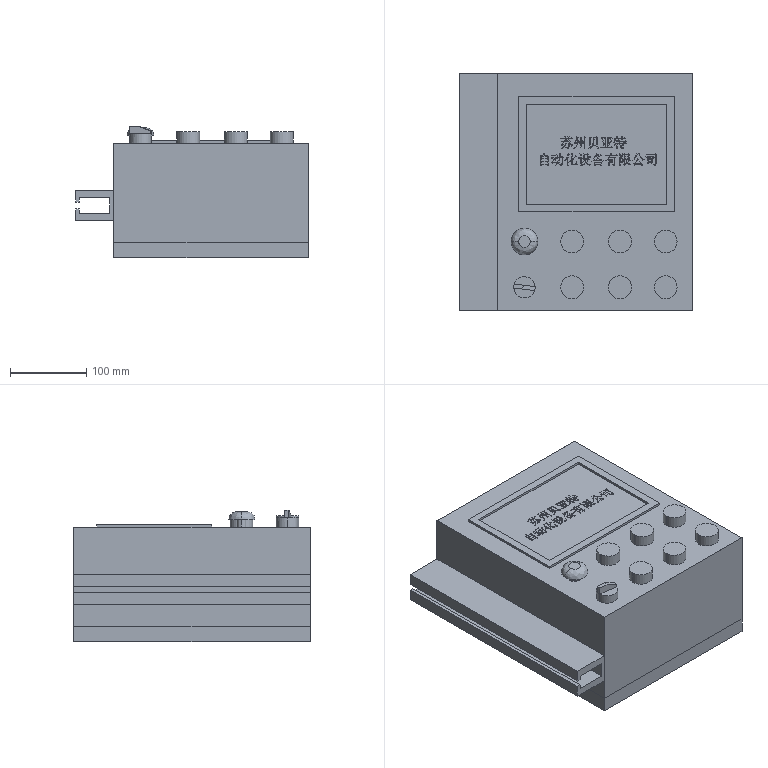Part | STEP file | Touch screen 2 | 2 solids | 673 faces | box 305 x 310 x 172 mm | volume 12316127 mm3 | plane 496 | spline 159 | cylinder 18 | commonest cylinder face diameters 30 x12 12 x2 15 x2 28 x2